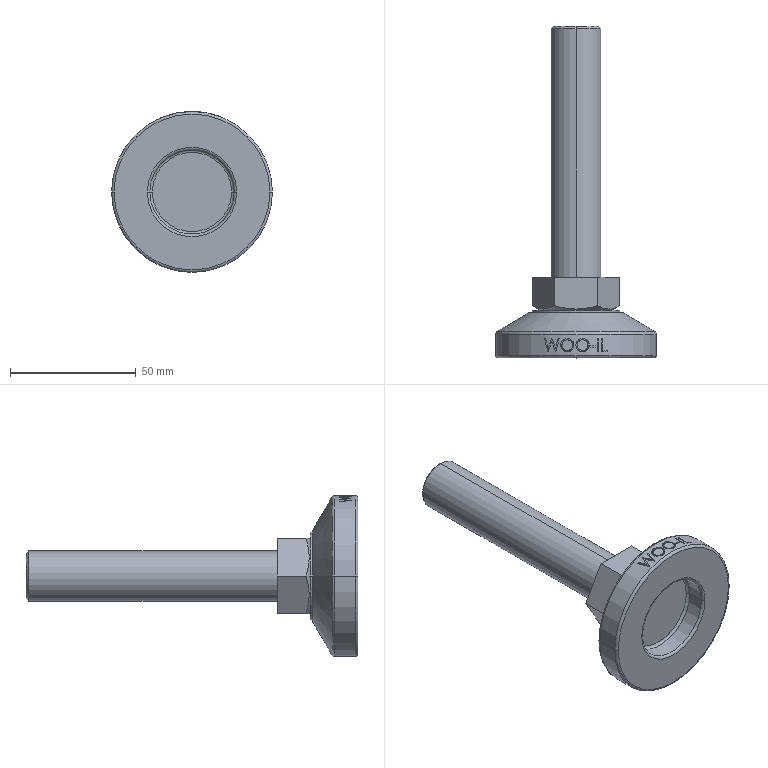Part | STEP file | MF64-M20-100_1 | 2 solids | 88 faces | box 64 x 132 x 64 mm | volume 83393 mm3 | plane 40 | cylinder 16 | spline 16 | torus 10 | cone 6 | commonest cylinder face diameters 64 x10 20 x2 33.6 x2 35 x2